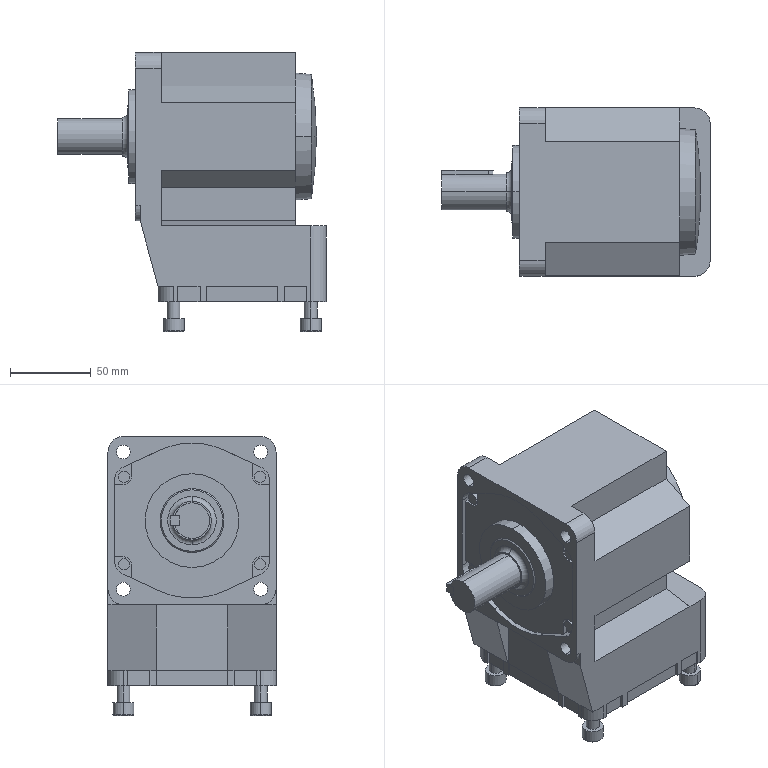Part | STEP file | 3 solids | 203 faces | box 166 x 104 x 172.5 mm | volume 1495766 mm3 | plane 128 | cylinder 59 | torus 10 | cone 4 | sphere 2 | commonest cylinder face diameters 7 x8 8 x8 8.5 x8 13 x8 19.2 x8 9.2 x4